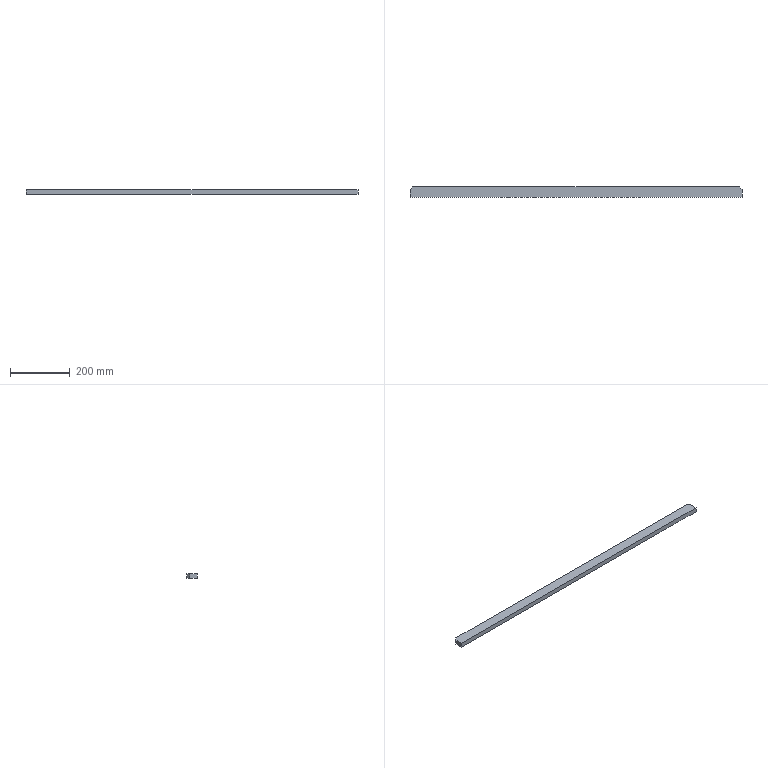Part | SolidWorks | features Chamfer 1, Extrusion 1 | 1 solid | 8 faces | box 1110 x 35 x 16 mm | volume 620000 mm3 | plane 8
STEP:
#1=CARTESIAN_POINT('',(1035.486,32.623,16.));
#2=VERTEX_POINT('',#1);
#3=CARTESIAN_POINT('',(-54.514,32.623,16.));
#4=VERTEX_POINT('',#3);
#5=CARTESIAN_POINT('',(1045.486,32.623,16.));
#6=DIRECTION('',(-1.,0.,0.));
#7=VECTOR('',#6,1000.);
#8=LINE('',#5,#7);
#9=EDGE_CURVE('',#2,#4,#8,.T.);
#10=ORIENTED_EDGE('',*,*,#9,.F.);
#11=CARTESIAN_POINT('',(1035.486,32.623,0.));
#12=VERTEX_POINT('',#11);
#13=CARTESIAN_POINT('',(1035.486,32.623,16.));
#14=DIRECTION('',(0.,0.,-1.));
#15=VECTOR('',#14,1000.);
#16=LINE('',#13,#15);
#17=EDGE_CURVE('',#2,#12,#16,.T.);
#18=ORIENTED_EDGE('',*,*,#17,.T.);
#19=CARTESIAN_POINT('',(-54.514,32.623,0.));
#20=VERTEX_POINT('',#19);
#21=CARTESIAN_POINT('',(1045.486,32.623,0.));
#22=DIRECTION('',(-1.,0.,0.));
#23=VECTOR('',#22,1000.);
#24=LINE('',#21,#23);
#25=EDGE_CURVE('',#12,#20,#24,.T.);
#26=ORIENTED_EDGE('',*,*,#25,.T.);
#27=CARTESIAN_POINT('',(-54.514,32.623,16.));
#28=DIRECTION('',(0.,0.,1.));
#29=VECTOR('',#28,1000.);
#30=LINE('',#27,#29);
#31=EDGE_CURVE('',#20,#4,#30,.T.);
#32=ORIENTED_EDGE('',*,*,#31,.T.);
#33=EDGE_LOOP('',(#10,#18,#26,#32));
#34=FACE_OUTER_BOUND('',#33,.T.);
#35=CARTESIAN_POINT('',(1045.486,32.623,16.));
#36=DIRECTION('',(0.,-1.,0.));
#37=DIRECTION('',(1.,0.,0.));
#38=AXIS2_PLACEMENT_3D('',#35,#36,#37);
#39=PLANE('',#38);
#40=ADVANCED_FACE('',(#34),#39,.F.);
#41=CARTESIAN_POINT('',(-64.514,22.623,16.));
#42=VERTEX_POINT('',#41);
#43=CARTESIAN_POINT('',(-64.514,-2.377,16.));
#44=VERTEX_POINT('',#43);
#45=CARTESIAN_POINT('',(-64.514,32.623,16.));
#46=DIRECTION('',(0.,-1.,0.));
#47=VECTOR('',#46,1000.);
#48=LINE('',#45,#47);
#49=EDGE_CURVE('',#42,#44,#48,.T.);
#50=ORIENTED_EDGE('',*,*,#49,.F.);
#51=CARTESIAN_POINT('',(-64.514,22.623,0.));
#52=VERTEX_POINT('',#51);
#53=CARTESIAN_POINT('',(-64.514,22.623,16.));
#54=DIRECTION('',(0.,0.,-1.));
#55=VECTOR('',#54,1000.);
#56=LINE('',#53,#55);
#57=EDGE_CURVE('',#42,#52,#56,.T.);
#58=ORIENTED_EDGE('',*,*,#57,.T.);
#59=CARTESIAN_POINT('',(-64.514,-2.377,0.));
#60=VERTEX_POINT('',#59);
#61=CARTESIAN_POINT('',(-64.514,32.623,0.));
#62=DIRECTION('',(0.,-1.,0.));
#63=VECTOR('',#62,1000.);
#64=LINE('',#61,#63);
#65=EDGE_CURVE('',#52,#60,#64,.T.);
#66=ORIENTED_EDGE('',*,*,#65,.T.);
#67=CARTESIAN_POINT('',(-64.514,-2.377,16.));
#68=DIRECTION('',(0.,0.,-1.));
#69=VECTOR('',#68,1000.);
#70=LINE('',#67,#69);
#71=EDGE_CURVE('',#44,#60,#70,.T.);
#72=ORIENTED_EDGE('',*,*,#71,.F.);
#73=EDGE_LOOP('',(#50,#58,#66,#72));
#74=FACE_OUTER_BOUND('',#73,.T.);
#75=CARTESIAN_POINT('',(-64.514,32.623,16.));
#76=DIRECTION('',(1.,0.,0.));
#77=DIRECTION('',(0.,0.,-1.));
#78=AXIS2_PLACEMENT_3D('',#75,#76,#77);
#79=PLANE('',#78);
#80=ADVANCED_FACE('',(#74),#79,.F.);
#81=CARTESIAN_POINT('',(1045.486,-2.377,0.));
#82=VERTEX_POINT('',#81);
#83=CARTESIAN_POINT('',(-64.514,-2.377,0.));
#84=DIRECTION('',(1.,0.,0.));
#85=VECTOR('',#84,1000.);
#86=LINE('',#83,#85);
#87=EDGE_CURVE('',#60,#82,#86,.T.);
#88=ORIENTED_EDGE('',*,*,#87,.T.);
#89=CARTESIAN_POINT('',(1045.486,-2.377,16.));
#90=VERTEX_POINT('',#89);
#91=CARTESIAN_POINT('',(1045.486,-2.377,16.));
#92=DIRECTION('',(0.,0.,-1.));
#93=VECTOR('',#92,1000.);
#94=LINE('',#91,#93);
#95=EDGE_CURVE('',#90,#82,#94,.T.);
#96=ORIENTED_EDGE('',*,*,#95,.F.);
#97=CARTESIAN_POINT('',(-64.514,-2.377,16.));
#98=DIRECTION('',(1.,0.,0.));
#99=VECTOR('',#98,1000.);
#100=LINE('',#97,#99);
#101=EDGE_CURVE('',#44,#90,#100,.T.);
#102=ORIENTED_EDGE('',*,*,#101,.F.);
#103=ORIENTED_EDGE('',*,*,#71,.T.);
#104=EDGE_LOOP('',(#88,#96,#102,#103));
#105=FACE_OUTER_BOUND('',#104,.T.);
#106=CARTESIAN_POINT('',(-64.514,-2.377,16.));
#107=DIRECTION('',(0.,1.,0.));
#108=DIRECTION('',(0.,0.,1.));
#109=AXIS2_PLACEMENT_3D('',#106,#107,#108);
#110=PLANE('',#109);
#111=ADVANCED_FACE('',(#105),#110,.F.);
#112=CARTESIAN_POINT('',(1045.486,22.623,0.));
#113=VERTEX_POINT('',#112);
#114=CARTESIAN_POINT('',(1045.486,-2.377,0.));
#115=DIRECTION('',(0.,1.,0.));
#116=VECTOR('',#115,1000.);
#117=LINE('',#114,#116);
#118=EDGE_CURVE('',#82,#113,#117,.T.);
#119=ORIENTED_EDGE('',*,*,#118,.T.);
#120=CARTESIAN_POINT('',(1045.486,22.623,16.));
#121=VERTEX_POINT('',#120);
#122=CARTESIAN_POINT('',(1045.486,22.623,16.));
#123=DIRECTION('',(0.,0.,1.));
#124=VECTOR('',#123,1000.);
#125=LINE('',#122,#124);
#126=EDGE_CURVE('',#113,#121,#125,.T.);
#127=ORIENTED_EDGE('',*,*,#126,.T.);
#128=CARTESIAN_POINT('',(1045.486,-2.377,16.));
#129=DIRECTION('',(0.,1.,0.));
#130=VECTOR('',#129,1000.);
#131=LINE('',#128,#130);
#132=EDGE_CURVE('',#90,#121,#131,.T.);
#133=ORIENTED_EDGE('',*,*,#132,.F.);
#134=ORIENTED_EDGE('',*,*,#95,.T.);
#135=EDGE_LOOP('',(#119,#127,#133,#134));
#136=FACE_OUTER_BOUND('',#135,.T.);
#137=CARTESIAN_POINT('',(1045.486,-2.377,16.));
#138=DIRECTION('',(-1.,0.,0.));
#139=DIRECTION('',(0.,0.,1.));
#140=AXIS2_PLACEMENT_3D('',#137,#138,#139);
#141=PLANE('',#140);
#142=ADVANCED_FACE('',(#136),#141,.F.);
#143=ORIENTED_EDGE('',*,*,#132,.T.);
#144=CARTESIAN_POINT('',(534.055,534.055,16.));
#145=DIRECTION('',(-0.7071,0.7071,0.));
#146=VECTOR('',#145,1000.);
#147=LINE('',#144,#146);
#148=EDGE_CURVE('',#121,#2,#147,.T.);
#149=ORIENTED_EDGE('',*,*,#148,.T.);
#150=ORIENTED_EDGE('',*,*,#9,.T.);
#151=CARTESIAN_POINT('',(-43.569,43.569,16.));
#152=DIRECTION('',(-0.7071,-0.7071,0.));
#153=VECTOR('',#152,1000.);
#154=LINE('',#151,#153);
#155=EDGE_CURVE('',#4,#42,#154,.T.);
#156=ORIENTED_EDGE('',*,*,#155,.T.);
#157=ORIENTED_EDGE('',*,*,#49,.T.);
#158=ORIENTED_EDGE('',*,*,#101,.T.);
#159=EDGE_LOOP('',(#143,#149,#150,#156,#157,#158));
#160=FACE_OUTER_BOUND('',#159,.T.);
#161=CARTESIAN_POINT('',(0.,0.,16.));
#162=DIRECTION('',(0.,0.,1.));
#163=DIRECTION('',(1.,0.,0.));
#164=AXIS2_PLACEMENT_3D('',#161,#162,#163);
#165=PLANE('',#164);
#166=ADVANCED_FACE('',(#160),#165,.T.);
#167=ORIENTED_EDGE('',*,*,#25,.F.);
#168=CARTESIAN_POINT('',(1035.486,32.623,0.));
#169=DIRECTION('',(0.7071,-0.7071,0.));
#170=VECTOR('',#169,1000.);
#171=LINE('',#168,#170);
#172=EDGE_CURVE('',#12,#113,#171,.T.);
#173=ORIENTED_EDGE('',*,*,#172,.T.);
#174=ORIENTED_EDGE('',*,*,#118,.F.);
#175=ORIENTED_EDGE('',*,*,#87,.F.);
#176=ORIENTED_EDGE('',*,*,#65,.F.);
#177=CARTESIAN_POINT('',(-64.514,22.623,0.));
#178=DIRECTION('',(0.7071,0.7071,0.));
#179=VECTOR('',#178,1000.);
#180=LINE('',#177,#179);
#181=EDGE_CURVE('',#52,#20,#180,.T.);
#182=ORIENTED_EDGE('',*,*,#181,.T.);
#183=EDGE_LOOP('',(#167,#173,#174,#175,#176,#182));
#184=FACE_OUTER_BOUND('',#183,.T.);
#185=CARTESIAN_POINT('',(0.,0.,0.));
#186=DIRECTION('',(0.,0.,1.));
#187=DIRECTION('',(1.,0.,0.));
#188=AXIS2_PLACEMENT_3D('',#185,#186,#187);
#189=PLANE('',#188);
#190=ADVANCED_FACE('',(#184),#189,.F.);
#191=ORIENTED_EDGE('',*,*,#148,.F.);
#192=ORIENTED_EDGE('',*,*,#126,.F.);
#193=ORIENTED_EDGE('',*,*,#172,.F.);
#194=ORIENTED_EDGE('',*,*,#17,.F.);
#195=EDGE_LOOP('',(#191,#192,#193,#194));
#196=FACE_OUTER_BOUND('',#195,.T.);
#197=CARTESIAN_POINT('',(1035.486,32.623,16.));
#198=DIRECTION('',(-0.7071,-0.7071,0.));
#199=DIRECTION('',(0.,0.,-1.));
#200=AXIS2_PLACEMENT_3D('',#197,#198,#199);
#201=PLANE('',#200);
#202=ADVANCED_FACE('',(#196),#201,.F.);
#203=ORIENTED_EDGE('',*,*,#155,.F.);
#204=ORIENTED_EDGE('',*,*,#31,.F.);
#205=ORIENTED_EDGE('',*,*,#181,.F.);
#206=ORIENTED_EDGE('',*,*,#57,.F.);
#207=EDGE_LOOP('',(#203,#204,#205,#206));
#208=FACE_OUTER_BOUND('',#207,.T.);
#209=CARTESIAN_POINT('',(-64.514,22.623,16.));
#210=DIRECTION('',(0.7071,-0.7071,0.));
#211=DIRECTION('',(0.,0.,-1.));
#212=AXIS2_PLACEMENT_3D('',#209,#210,#211);
#213=PLANE('',#212);
#214=ADVANCED_FACE('',(#208),#213,.F.);
#215=CLOSED_SHELL('',(#40,#80,#111,#142,#166,#190,#202,#214));
#216=MANIFOLD_SOLID_BREP('',#215);
#217=CARTESIAN_POINT('',(0.,0.,0.));
#218=DIRECTION('',(0.,0.,1.));
#219=DIRECTION('',(1.,0.,0.));
#220=AXIS2_PLACEMENT_3D('',#217,#218,#219);
#221=(LENGTH_UNIT()NAMED_UNIT(*)SI_UNIT(.MILLI.,.METRE.));
#222=UNCERTAINTY_MEASURE_WITH_UNIT(LENGTH_MEASURE(0.00001),#221,'','');
#223=(NAMED_UNIT(*)PLANE_ANGLE_UNIT()SI_UNIT($,.RADIAN.));
#224=(NAMED_UNIT(*)SI_UNIT($,.STERADIAN.)SOLID_ANGLE_UNIT());
#225=(GEOMETRIC_REPRESENTATION_CONTEXT(3)GLOBAL_UNCERTAINTY_ASSIGNED_CONTEXT((#222))GLOBAL_UNIT_ASSIGNED_CONTEXT((#221,#223,#224))REPRESENTATION_CONTEXT('',''));
#226=ADVANCED_BREP_SHAPE_REPRESENTATION('',(#216,#220),#225);